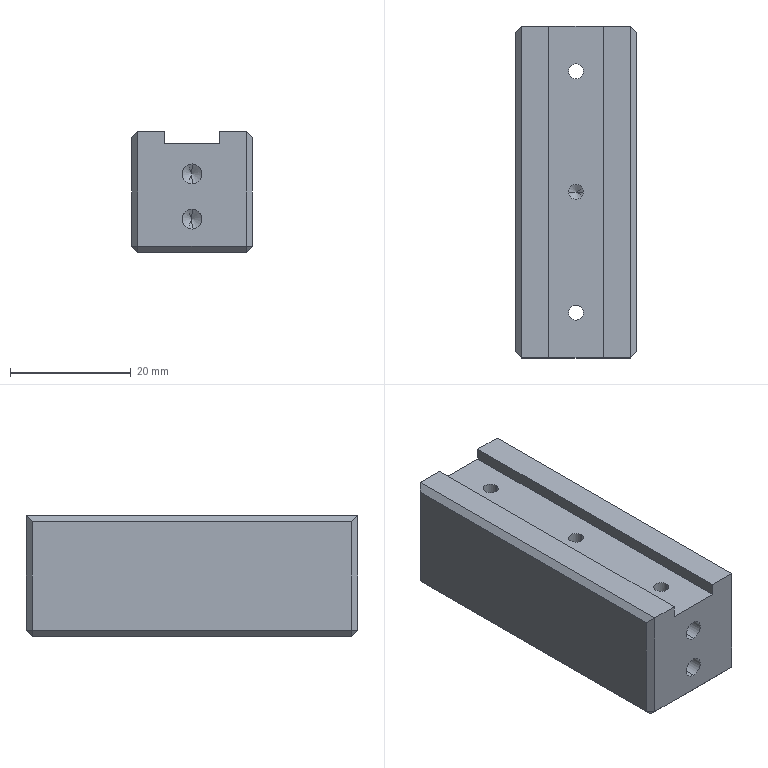Part | SolidWorks | features HoleWzd 3, Chamfer 1, Extrusion 1, ICE 1 | 1 solid | 51 faces | box 20 x 55 x 20 mm | volume 20279 mm3 | plane 24 | cylinder 16 | cone 11 | commonest cylinder face diameters 2.5 x6 3.3 x6 4.2 x4